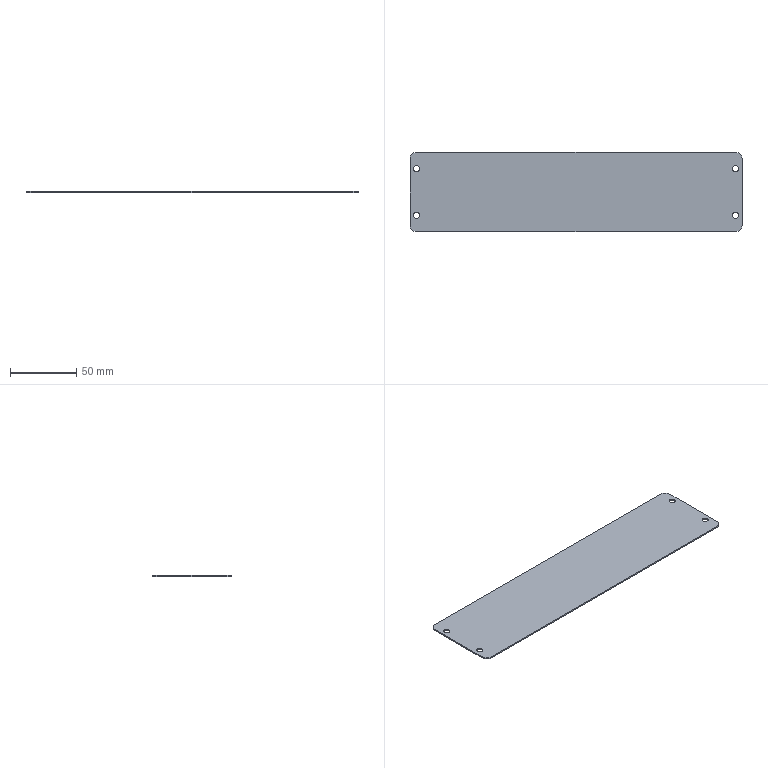Part | SolidWorks | features BreakCorner 1, FlatPattern 1, HoleWzd 1, SMBaseFlange 1, SheetMetal 1 | 1 solid | 18 faces | box 250 x 60 x 1 mm | volume 14915 mm3 | cylinder 12 | plane 6 | commonest cylinder face diameters 4.5 x8 10 x4
STEP:
#1=CARTESIAN_POINT('',(122.25,17.5,0.));
#2=VERTEX_POINT('',#1);
#3=CARTESIAN_POINT('',(117.75,17.5,0.));
#4=VERTEX_POINT('',#3);
#5=CARTESIAN_POINT('',(120.,17.5,0.));
#6=DIRECTION('',(0.,0.,-1.));
#7=DIRECTION('',(-1.,0.,0.));
#8=AXIS2_PLACEMENT_3D('',#5,#6,#7);
#9=CIRCLE('',#8,2.25);
#10=EDGE_CURVE('',#2,#4,#9,.T.);
#11=ORIENTED_EDGE('',*,*,#10,.F.);
#12=CARTESIAN_POINT('',(122.25,17.5,-1.));
#13=VERTEX_POINT('',#12);
#14=CARTESIAN_POINT('',(122.25,17.5,-1.));
#15=DIRECTION('',(0.,0.,-1.));
#16=VECTOR('',#15,1000.);
#17=LINE('',#14,#16);
#18=EDGE_CURVE('',#2,#13,#17,.T.);
#19=ORIENTED_EDGE('',*,*,#18,.T.);
#20=CARTESIAN_POINT('',(117.75,17.5,-1.));
#21=VERTEX_POINT('',#20);
#22=CARTESIAN_POINT('',(120.,17.5,-1.));
#23=DIRECTION('',(0.,0.,-1.));
#24=DIRECTION('',(-1.,0.,0.));
#25=AXIS2_PLACEMENT_3D('',#22,#23,#24);
#26=CIRCLE('',#25,2.25);
#27=EDGE_CURVE('',#13,#21,#26,.T.);
#28=ORIENTED_EDGE('',*,*,#27,.T.);
#29=CARTESIAN_POINT('',(117.75,17.5,-1.));
#30=DIRECTION('',(0.,0.,-1.));
#31=VECTOR('',#30,1000.);
#32=LINE('',#29,#31);
#33=EDGE_CURVE('',#4,#21,#32,.T.);
#34=ORIENTED_EDGE('',*,*,#33,.F.);
#35=EDGE_LOOP('',(#11,#19,#28,#34));
#36=FACE_OUTER_BOUND('',#35,.T.);
#37=CARTESIAN_POINT('',(120.,17.5,-1.));
#38=DIRECTION('',(0.,0.,-1.));
#39=DIRECTION('',(-1.,0.,0.));
#40=AXIS2_PLACEMENT_3D('',#37,#38,#39);
#41=CYLINDRICAL_SURFACE('',#40,2.25);
#42=ADVANCED_FACE('',(#36),#41,.F.);
#43=CARTESIAN_POINT('',(122.25,-17.5,0.));
#44=VERTEX_POINT('',#43);
#45=CARTESIAN_POINT('',(117.75,-17.5,0.));
#46=VERTEX_POINT('',#45);
#47=CARTESIAN_POINT('',(120.,-17.5,0.));
#48=DIRECTION('',(0.,0.,-1.));
#49=DIRECTION('',(-1.,0.,0.));
#50=AXIS2_PLACEMENT_3D('',#47,#48,#49);
#51=CIRCLE('',#50,2.25);
#52=EDGE_CURVE('',#44,#46,#51,.T.);
#53=ORIENTED_EDGE('',*,*,#52,.F.);
#54=CARTESIAN_POINT('',(122.25,-17.5,-1.));
#55=VERTEX_POINT('',#54);
#56=CARTESIAN_POINT('',(122.25,-17.5,-1.));
#57=DIRECTION('',(0.,0.,-1.));
#58=VECTOR('',#57,1000.);
#59=LINE('',#56,#58);
#60=EDGE_CURVE('',#44,#55,#59,.T.);
#61=ORIENTED_EDGE('',*,*,#60,.T.);
#62=CARTESIAN_POINT('',(117.75,-17.5,-1.));
#63=VERTEX_POINT('',#62);
#64=CARTESIAN_POINT('',(120.,-17.5,-1.));
#65=DIRECTION('',(0.,0.,-1.));
#66=DIRECTION('',(-1.,0.,0.));
#67=AXIS2_PLACEMENT_3D('',#64,#65,#66);
#68=CIRCLE('',#67,2.25);
#69=EDGE_CURVE('',#55,#63,#68,.T.);
#70=ORIENTED_EDGE('',*,*,#69,.T.);
#71=CARTESIAN_POINT('',(117.75,-17.5,-1.));
#72=DIRECTION('',(0.,0.,-1.));
#73=VECTOR('',#72,1000.);
#74=LINE('',#71,#73);
#75=EDGE_CURVE('',#46,#63,#74,.T.);
#76=ORIENTED_EDGE('',*,*,#75,.F.);
#77=EDGE_LOOP('',(#53,#61,#70,#76));
#78=FACE_OUTER_BOUND('',#77,.T.);
#79=CARTESIAN_POINT('',(120.,-17.5,-1.));
#80=DIRECTION('',(0.,0.,-1.));
#81=DIRECTION('',(-1.,0.,0.));
#82=AXIS2_PLACEMENT_3D('',#79,#80,#81);
#83=CYLINDRICAL_SURFACE('',#82,2.25);
#84=ADVANCED_FACE('',(#78),#83,.F.);
#85=CARTESIAN_POINT('',(-117.75,17.5,0.));
#86=VERTEX_POINT('',#85);
#87=CARTESIAN_POINT('',(-122.25,17.5,0.));
#88=VERTEX_POINT('',#87);
#89=CARTESIAN_POINT('',(-120.,17.5,0.));
#90=DIRECTION('',(0.,0.,-1.));
#91=DIRECTION('',(-1.,0.,0.));
#92=AXIS2_PLACEMENT_3D('',#89,#90,#91);
#93=CIRCLE('',#92,2.25);
#94=EDGE_CURVE('',#86,#88,#93,.T.);
#95=ORIENTED_EDGE('',*,*,#94,.F.);
#96=CARTESIAN_POINT('',(-117.75,17.5,-1.));
#97=VERTEX_POINT('',#96);
#98=CARTESIAN_POINT('',(-117.75,17.5,-1.));
#99=DIRECTION('',(0.,0.,-1.));
#100=VECTOR('',#99,1000.);
#101=LINE('',#98,#100);
#102=EDGE_CURVE('',#86,#97,#101,.T.);
#103=ORIENTED_EDGE('',*,*,#102,.T.);
#104=CARTESIAN_POINT('',(-122.25,17.5,-1.));
#105=VERTEX_POINT('',#104);
#106=CARTESIAN_POINT('',(-120.,17.5,-1.));
#107=DIRECTION('',(0.,0.,-1.));
#108=DIRECTION('',(-1.,0.,0.));
#109=AXIS2_PLACEMENT_3D('',#106,#107,#108);
#110=CIRCLE('',#109,2.25);
#111=EDGE_CURVE('',#97,#105,#110,.T.);
#112=ORIENTED_EDGE('',*,*,#111,.T.);
#113=CARTESIAN_POINT('',(-122.25,17.5,-1.));
#114=DIRECTION('',(0.,0.,-1.));
#115=VECTOR('',#114,1000.);
#116=LINE('',#113,#115);
#117=EDGE_CURVE('',#88,#105,#116,.T.);
#118=ORIENTED_EDGE('',*,*,#117,.F.);
#119=EDGE_LOOP('',(#95,#103,#112,#118));
#120=FACE_OUTER_BOUND('',#119,.T.);
#121=CARTESIAN_POINT('',(-120.,17.5,-1.));
#122=DIRECTION('',(0.,0.,-1.));
#123=DIRECTION('',(-1.,0.,0.));
#124=AXIS2_PLACEMENT_3D('',#121,#122,#123);
#125=CYLINDRICAL_SURFACE('',#124,2.25);
#126=ADVANCED_FACE('',(#120),#125,.F.);
#127=CARTESIAN_POINT('',(-117.75,-17.5,0.));
#128=VERTEX_POINT('',#127);
#129=CARTESIAN_POINT('',(-122.25,-17.5,0.));
#130=VERTEX_POINT('',#129);
#131=CARTESIAN_POINT('',(-120.,-17.5,0.));
#132=DIRECTION('',(0.,0.,-1.));
#133=DIRECTION('',(-1.,0.,0.));
#134=AXIS2_PLACEMENT_3D('',#131,#132,#133);
#135=CIRCLE('',#134,2.25);
#136=EDGE_CURVE('',#128,#130,#135,.T.);
#137=ORIENTED_EDGE('',*,*,#136,.F.);
#138=CARTESIAN_POINT('',(-117.75,-17.5,-1.));
#139=VERTEX_POINT('',#138);
#140=CARTESIAN_POINT('',(-117.75,-17.5,-1.));
#141=DIRECTION('',(0.,0.,-1.));
#142=VECTOR('',#141,1000.);
#143=LINE('',#140,#142);
#144=EDGE_CURVE('',#128,#139,#143,.T.);
#145=ORIENTED_EDGE('',*,*,#144,.T.);
#146=CARTESIAN_POINT('',(-122.25,-17.5,-1.));
#147=VERTEX_POINT('',#146);
#148=CARTESIAN_POINT('',(-120.,-17.5,-1.));
#149=DIRECTION('',(0.,0.,-1.));
#150=DIRECTION('',(-1.,0.,0.));
#151=AXIS2_PLACEMENT_3D('',#148,#149,#150);
#152=CIRCLE('',#151,2.25);
#153=EDGE_CURVE('',#139,#147,#152,.T.);
#154=ORIENTED_EDGE('',*,*,#153,.T.);
#155=CARTESIAN_POINT('',(-122.25,-17.5,-1.));
#156=DIRECTION('',(0.,0.,-1.));
#157=VECTOR('',#156,1000.);
#158=LINE('',#155,#157);
#159=EDGE_CURVE('',#130,#147,#158,.T.);
#160=ORIENTED_EDGE('',*,*,#159,.F.);
#161=EDGE_LOOP('',(#137,#145,#154,#160));
#162=FACE_OUTER_BOUND('',#161,.T.);
#163=CARTESIAN_POINT('',(-120.,-17.5,-1.));
#164=DIRECTION('',(0.,0.,-1.));
#165=DIRECTION('',(-1.,0.,0.));
#166=AXIS2_PLACEMENT_3D('',#163,#164,#165);
#167=CYLINDRICAL_SURFACE('',#166,2.25);
#168=ADVANCED_FACE('',(#162),#167,.F.);
#169=CARTESIAN_POINT('',(125.,-25.,-1.));
#170=VERTEX_POINT('',#169);
#171=CARTESIAN_POINT('',(125.,25.,-1.));
#172=VERTEX_POINT('',#171);
#173=CARTESIAN_POINT('',(125.,-30.,-1.));
#174=DIRECTION('',(0.,1.,0.));
#175=VECTOR('',#174,1000.);
#176=LINE('',#173,#175);
#177=EDGE_CURVE('',#170,#172,#176,.T.);
#178=ORIENTED_EDGE('',*,*,#177,.T.);
#179=CARTESIAN_POINT('',(125.,25.,0.));
#180=VERTEX_POINT('',#179);
#181=CARTESIAN_POINT('',(125.,25.,-1.));
#182=DIRECTION('',(0.,0.,1.));
#183=VECTOR('',#182,1000.);
#184=LINE('',#181,#183);
#185=EDGE_CURVE('',#172,#180,#184,.T.);
#186=ORIENTED_EDGE('',*,*,#185,.T.);
#187=CARTESIAN_POINT('',(125.,-25.,0.));
#188=VERTEX_POINT('',#187);
#189=CARTESIAN_POINT('',(125.,-30.,0.));
#190=DIRECTION('',(0.,1.,0.));
#191=VECTOR('',#190,1000.);
#192=LINE('',#189,#191);
#193=EDGE_CURVE('',#188,#180,#192,.T.);
#194=ORIENTED_EDGE('',*,*,#193,.F.);
#195=CARTESIAN_POINT('',(125.,-25.,-1.));
#196=DIRECTION('',(0.,0.,-1.));
#197=VECTOR('',#196,1000.);
#198=LINE('',#195,#197);
#199=EDGE_CURVE('',#188,#170,#198,.T.);
#200=ORIENTED_EDGE('',*,*,#199,.T.);
#201=EDGE_LOOP('',(#178,#186,#194,#200));
#202=FACE_OUTER_BOUND('',#201,.T.);
#203=CARTESIAN_POINT('',(125.,-30.,-1.));
#204=DIRECTION('',(1.,0.,0.));
#205=DIRECTION('',(0.,0.,-1.));
#206=AXIS2_PLACEMENT_3D('',#203,#204,#205);
#207=PLANE('',#206);
#208=ADVANCED_FACE('',(#202),#207,.T.);
#209=CARTESIAN_POINT('',(-120.,-30.,0.));
#210=VERTEX_POINT('',#209);
#211=CARTESIAN_POINT('',(120.,-30.,0.));
#212=VERTEX_POINT('',#211);
#213=CARTESIAN_POINT('',(-125.,-30.,0.));
#214=DIRECTION('',(1.,0.,0.));
#215=VECTOR('',#214,1000.);
#216=LINE('',#213,#215);
#217=EDGE_CURVE('',#210,#212,#216,.T.);
#218=ORIENTED_EDGE('',*,*,#217,.F.);
#219=CARTESIAN_POINT('',(-120.,-30.,-1.));
#220=VERTEX_POINT('',#219);
#221=CARTESIAN_POINT('',(-120.,-30.,-1.));
#222=DIRECTION('',(0.,0.,-1.));
#223=VECTOR('',#222,1000.);
#224=LINE('',#221,#223);
#225=EDGE_CURVE('',#210,#220,#224,.T.);
#226=ORIENTED_EDGE('',*,*,#225,.T.);
#227=CARTESIAN_POINT('',(120.,-30.,-1.));
#228=VERTEX_POINT('',#227);
#229=CARTESIAN_POINT('',(-125.,-30.,-1.));
#230=DIRECTION('',(1.,0.,0.));
#231=VECTOR('',#230,1000.);
#232=LINE('',#229,#231);
#233=EDGE_CURVE('',#220,#228,#232,.T.);
#234=ORIENTED_EDGE('',*,*,#233,.T.);
#235=CARTESIAN_POINT('',(120.,-30.,-1.));
#236=DIRECTION('',(0.,0.,1.));
#237=VECTOR('',#236,1000.);
#238=LINE('',#235,#237);
#239=EDGE_CURVE('',#228,#212,#238,.T.);
#240=ORIENTED_EDGE('',*,*,#239,.T.);
#241=EDGE_LOOP('',(#218,#226,#234,#240));
#242=FACE_OUTER_BOUND('',#241,.T.);
#243=CARTESIAN_POINT('',(-125.,-30.,-1.));
#244=DIRECTION('',(0.,-1.,0.));
#245=DIRECTION('',(0.,0.,-1.));
#246=AXIS2_PLACEMENT_3D('',#243,#244,#245);
#247=PLANE('',#246);
#248=ADVANCED_FACE('',(#242),#247,.T.);
#249=CARTESIAN_POINT('',(-125.,25.,0.));
#250=VERTEX_POINT('',#249);
#251=CARTESIAN_POINT('',(-125.,-25.,0.));
#252=VERTEX_POINT('',#251);
#253=CARTESIAN_POINT('',(-125.,-30.,0.));
#254=DIRECTION('',(0.,-1.,0.));
#255=VECTOR('',#254,1000.);
#256=LINE('',#253,#255);
#257=EDGE_CURVE('',#250,#252,#256,.T.);
#258=ORIENTED_EDGE('',*,*,#257,.F.);
#259=CARTESIAN_POINT('',(-125.,25.,-1.));
#260=VERTEX_POINT('',#259);
#261=CARTESIAN_POINT('',(-125.,25.,-1.));
#262=DIRECTION('',(0.,0.,-1.));
#263=VECTOR('',#262,1000.);
#264=LINE('',#261,#263);
#265=EDGE_CURVE('',#250,#260,#264,.T.);
#266=ORIENTED_EDGE('',*,*,#265,.T.);
#267=CARTESIAN_POINT('',(-125.,-25.,-1.));
#268=VERTEX_POINT('',#267);
#269=CARTESIAN_POINT('',(-125.,-30.,-1.));
#270=DIRECTION('',(0.,-1.,0.));
#271=VECTOR('',#270,1000.);
#272=LINE('',#269,#271);
#273=EDGE_CURVE('',#260,#268,#272,.T.);
#274=ORIENTED_EDGE('',*,*,#273,.T.);
#275=CARTESIAN_POINT('',(-125.,-25.,-1.));
#276=DIRECTION('',(0.,0.,1.));
#277=VECTOR('',#276,1000.);
#278=LINE('',#275,#277);
#279=EDGE_CURVE('',#268,#252,#278,.T.);
#280=ORIENTED_EDGE('',*,*,#279,.T.);
#281=EDGE_LOOP('',(#258,#266,#274,#280));
#282=FACE_OUTER_BOUND('',#281,.T.);
#283=CARTESIAN_POINT('',(-125.,-30.,-1.));
#284=DIRECTION('',(-1.,0.,0.));
#285=DIRECTION('',(0.,0.,1.));
#286=AXIS2_PLACEMENT_3D('',#283,#284,#285);
#287=PLANE('',#286);
#288=ADVANCED_FACE('',(#282),#287,.T.);
#289=CARTESIAN_POINT('',(120.,30.,0.));
#290=VERTEX_POINT('',#289);
#291=CARTESIAN_POINT('',(-120.,30.,0.));
#292=VERTEX_POINT('',#291);
#293=CARTESIAN_POINT('',(-125.,30.,0.));
#294=DIRECTION('',(-1.,0.,0.));
#295=VECTOR('',#294,1000.);
#296=LINE('',#293,#295);
#297=EDGE_CURVE('',#290,#292,#296,.T.);
#298=ORIENTED_EDGE('',*,*,#297,.F.);
#299=CARTESIAN_POINT('',(120.,30.,-1.));
#300=VERTEX_POINT('',#299);
#301=CARTESIAN_POINT('',(120.,30.,-1.));
#302=DIRECTION('',(0.,0.,-1.));
#303=VECTOR('',#302,1000.);
#304=LINE('',#301,#303);
#305=EDGE_CURVE('',#290,#300,#304,.T.);
#306=ORIENTED_EDGE('',*,*,#305,.T.);
#307=CARTESIAN_POINT('',(-120.,30.,-1.));
#308=VERTEX_POINT('',#307);
#309=CARTESIAN_POINT('',(-125.,30.,-1.));
#310=DIRECTION('',(-1.,0.,0.));
#311=VECTOR('',#310,1000.);
#312=LINE('',#309,#311);
#313=EDGE_CURVE('',#300,#308,#312,.T.);
#314=ORIENTED_EDGE('',*,*,#313,.T.);
#315=CARTESIAN_POINT('',(-120.,30.,-1.));
#316=DIRECTION('',(0.,0.,1.));
#317=VECTOR('',#316,1000.);
#318=LINE('',#315,#317);
#319=EDGE_CURVE('',#308,#292,#318,.T.);
#320=ORIENTED_EDGE('',*,*,#319,.T.);
#321=EDGE_LOOP('',(#298,#306,#314,#320));
#322=FACE_OUTER_BOUND('',#321,.T.);
#323=CARTESIAN_POINT('',(-125.,30.,-1.));
#324=DIRECTION('',(0.,1.,0.));
#325=DIRECTION('',(0.,0.,1.));
#326=AXIS2_PLACEMENT_3D('',#323,#324,#325);
#327=PLANE('',#326);
#328=ADVANCED_FACE('',(#322),#327,.T.);
#329=CARTESIAN_POINT('',(120.,17.5,-1.));
#330=DIRECTION('',(0.,0.,-1.));
#331=DIRECTION('',(-1.,0.,0.));
#332=AXIS2_PLACEMENT_3D('',#329,#330,#331);
#333=CIRCLE('',#332,2.25);
#334=EDGE_CURVE('',#21,#13,#333,.T.);
#335=ORIENTED_EDGE('',*,*,#334,.F.);
#336=ORIENTED_EDGE('',*,*,#27,.F.);
#337=EDGE_LOOP('',(#335,#336));
#338=FACE_BOUND('',#337,.T.);
#339=CARTESIAN_POINT('',(120.,-17.5,-1.));
#340=DIRECTION('',(0.,0.,-1.));
#341=DIRECTION('',(-1.,0.,0.));
#342=AXIS2_PLACEMENT_3D('',#339,#340,#341);
#343=CIRCLE('',#342,2.25);
#344=EDGE_CURVE('',#63,#55,#343,.T.);
#345=ORIENTED_EDGE('',*,*,#344,.F.);
#346=ORIENTED_EDGE('',*,*,#69,.F.);
#347=EDGE_LOOP('',(#345,#346));
#348=FACE_BOUND('',#347,.T.);
#349=CARTESIAN_POINT('',(-120.,17.5,-1.));
#350=DIRECTION('',(0.,0.,-1.));
#351=DIRECTION('',(-1.,0.,0.));
#352=AXIS2_PLACEMENT_3D('',#349,#350,#351);
#353=CIRCLE('',#352,2.25);
#354=EDGE_CURVE('',#105,#97,#353,.T.);
#355=ORIENTED_EDGE('',*,*,#354,.F.);
#356=ORIENTED_EDGE('',*,*,#111,.F.);
#357=EDGE_LOOP('',(#355,#356));
#358=FACE_BOUND('',#357,.T.);
#359=CARTESIAN_POINT('',(-120.,-17.5,-1.));
#360=DIRECTION('',(0.,0.,-1.));
#361=DIRECTION('',(-1.,0.,0.));
#362=AXIS2_PLACEMENT_3D('',#359,#360,#361);
#363=CIRCLE('',#362,2.25);
#364=EDGE_CURVE('',#147,#139,#363,.T.);
#365=ORIENTED_EDGE('',*,*,#364,.F.);
#366=ORIENTED_EDGE('',*,*,#153,.F.);
#367=EDGE_LOOP('',(#365,#366));
#368=FACE_BOUND('',#367,.T.);
#369=ORIENTED_EDGE('',*,*,#313,.F.);
#370=CARTESIAN_POINT('',(120.,25.,-1.));
#371=DIRECTION('',(0.,0.,-1.));
#372=DIRECTION('',(-1.,0.,0.));
#373=AXIS2_PLACEMENT_3D('',#370,#371,#372);
#374=CIRCLE('',#373,5.);
#375=EDGE_CURVE('',#300,#172,#374,.T.);
#376=ORIENTED_EDGE('',*,*,#375,.T.);
#377=ORIENTED_EDGE('',*,*,#177,.F.);
#378=CARTESIAN_POINT('',(120.,-25.,-1.));
#379=DIRECTION('',(0.,0.,-1.));
#380=DIRECTION('',(-1.,0.,0.));
#381=AXIS2_PLACEMENT_3D('',#378,#379,#380);
#382=CIRCLE('',#381,5.);
#383=EDGE_CURVE('',#170,#228,#382,.T.);
#384=ORIENTED_EDGE('',*,*,#383,.T.);
#385=ORIENTED_EDGE('',*,*,#233,.F.);
#386=CARTESIAN_POINT('',(-120.,-25.,-1.));
#387=DIRECTION('',(0.,0.,-1.));
#388=DIRECTION('',(-1.,0.,0.));
#389=AXIS2_PLACEMENT_3D('',#386,#387,#388);
#390=CIRCLE('',#389,5.);
#391=EDGE_CURVE('',#220,#268,#390,.T.);
#392=ORIENTED_EDGE('',*,*,#391,.T.);
#393=ORIENTED_EDGE('',*,*,#273,.F.);
#394=CARTESIAN_POINT('',(-120.,25.,-1.));
#395=DIRECTION('',(0.,0.,-1.));
#396=DIRECTION('',(-1.,0.,0.));
#397=AXIS2_PLACEMENT_3D('',#394,#395,#396);
#398=CIRCLE('',#397,5.);
#399=EDGE_CURVE('',#260,#308,#398,.T.);
#400=ORIENTED_EDGE('',*,*,#399,.T.);
#401=EDGE_LOOP('',(#369,#376,#377,#384,#385,#392,#393,#400));
#402=FACE_OUTER_BOUND('',#401,.T.);
#403=CARTESIAN_POINT('',(0.,0.,-1.));
#404=DIRECTION('',(0.,0.,-1.));
#405=DIRECTION('',(-1.,0.,0.));
#406=AXIS2_PLACEMENT_3D('',#403,#404,#405);
#407=PLANE('',#406);
#408=ADVANCED_FACE('',(#338,#348,#358,#368,#402),#407,.T.);
#409=CARTESIAN_POINT('',(120.,17.5,0.));
#410=DIRECTION('',(0.,0.,-1.));
#411=DIRECTION('',(-1.,0.,0.));
#412=AXIS2_PLACEMENT_3D('',#409,#410,#411);
#413=CIRCLE('',#412,2.25);
#414=EDGE_CURVE('',#4,#2,#413,.T.);
#415=ORIENTED_EDGE('',*,*,#414,.T.);
#416=ORIENTED_EDGE('',*,*,#10,.T.);
#417=EDGE_LOOP('',(#415,#416));
#418=FACE_BOUND('',#417,.T.);
#419=CARTESIAN_POINT('',(120.,-17.5,0.));
#420=DIRECTION('',(0.,0.,-1.));
#421=DIRECTION('',(-1.,0.,0.));
#422=AXIS2_PLACEMENT_3D('',#419,#420,#421);
#423=CIRCLE('',#422,2.25);
#424=EDGE_CURVE('',#46,#44,#423,.T.);
#425=ORIENTED_EDGE('',*,*,#424,.T.);
#426=ORIENTED_EDGE('',*,*,#52,.T.);
#427=EDGE_LOOP('',(#425,#426));
#428=FACE_BOUND('',#427,.T.);
#429=CARTESIAN_POINT('',(-120.,17.5,0.));
#430=DIRECTION('',(0.,0.,-1.));
#431=DIRECTION('',(-1.,0.,0.));
#432=AXIS2_PLACEMENT_3D('',#429,#430,#431);
#433=CIRCLE('',#432,2.25);
#434=EDGE_CURVE('',#88,#86,#433,.T.);
#435=ORIENTED_EDGE('',*,*,#434,.T.);
#436=ORIENTED_EDGE('',*,*,#94,.T.);
#437=EDGE_LOOP('',(#435,#436));
#438=FACE_BOUND('',#437,.T.);
#439=CARTESIAN_POINT('',(-120.,-17.5,0.));
#440=DIRECTION('',(0.,0.,-1.));
#441=DIRECTION('',(-1.,0.,0.));
#442=AXIS2_PLACEMENT_3D('',#439,#440,#441);
#443=CIRCLE('',#442,2.25);
#444=EDGE_CURVE('',#130,#128,#443,.T.);
#445=ORIENTED_EDGE('',*,*,#444,.T.);
#446=ORIENTED_EDGE('',*,*,#136,.T.);
#447=EDGE_LOOP('',(#445,#446));
#448=FACE_BOUND('',#447,.T.);
#449=ORIENTED_EDGE('',*,*,#193,.T.);
#450=CARTESIAN_POINT('',(120.,25.,0.));
#451=DIRECTION('',(0.,0.,1.));
#452=DIRECTION('',(-1.,0.,0.));
#453=AXIS2_PLACEMENT_3D('',#450,#451,#452);
#454=CIRCLE('',#453,5.);
#455=EDGE_CURVE('',#180,#290,#454,.T.);
#456=ORIENTED_EDGE('',*,*,#455,.T.);
#457=ORIENTED_EDGE('',*,*,#297,.T.);
#458=CARTESIAN_POINT('',(-120.,25.,0.));
#459=DIRECTION('',(0.,0.,1.));
#460=DIRECTION('',(-1.,0.,0.));
#461=AXIS2_PLACEMENT_3D('',#458,#459,#460);
#462=CIRCLE('',#461,5.);
#463=EDGE_CURVE('',#292,#250,#462,.T.);
#464=ORIENTED_EDGE('',*,*,#463,.T.);
#465=ORIENTED_EDGE('',*,*,#257,.T.);
#466=CARTESIAN_POINT('',(-120.,-25.,0.));
#467=DIRECTION('',(0.,0.,1.));
#468=DIRECTION('',(-1.,0.,0.));
#469=AXIS2_PLACEMENT_3D('',#466,#467,#468);
#470=CIRCLE('',#469,5.);
#471=EDGE_CURVE('',#252,#210,#470,.T.);
#472=ORIENTED_EDGE('',*,*,#471,.T.);
#473=ORIENTED_EDGE('',*,*,#217,.T.);
#474=CARTESIAN_POINT('',(120.,-25.,0.));
#475=DIRECTION('',(0.,0.,1.));
#476=DIRECTION('',(-1.,0.,0.));
#477=AXIS2_PLACEMENT_3D('',#474,#475,#476);
#478=CIRCLE('',#477,5.);
#479=EDGE_CURVE('',#212,#188,#478,.T.);
#480=ORIENTED_EDGE('',*,*,#479,.T.);
#481=EDGE_LOOP('',(#449,#456,#457,#464,#465,#472,#473,#480));
#482=FACE_OUTER_BOUND('',#481,.T.);
#483=CARTESIAN_POINT('',(0.,0.,0.));
#484=DIRECTION('',(0.,0.,-1.));
#485=DIRECTION('',(-1.,0.,0.));
#486=AXIS2_PLACEMENT_3D('',#483,#484,#485);
#487=PLANE('',#486);
#488=ADVANCED_FACE('',(#418,#428,#438,#448,#482),#487,.F.);
#489=ORIENTED_EDGE('',*,*,#144,.F.);
#490=ORIENTED_EDGE('',*,*,#444,.F.);
#491=ORIENTED_EDGE('',*,*,#159,.T.);
#492=ORIENTED_EDGE('',*,*,#364,.T.);
#493=EDGE_LOOP('',(#489,#490,#491,#492));
#494=FACE_OUTER_BOUND('',#493,.T.);
#495=CARTESIAN_POINT('',(-120.,-17.5,-1.));
#496=DIRECTION('',(0.,0.,-1.));
#497=DIRECTION('',(-1.,0.,0.));
#498=AXIS2_PLACEMENT_3D('',#495,#496,#497);
#499=CYLINDRICAL_SURFACE('',#498,2.25);
#500=ADVANCED_FACE('',(#494),#499,.F.);
#501=ORIENTED_EDGE('',*,*,#102,.F.);
#502=ORIENTED_EDGE('',*,*,#434,.F.);
#503=ORIENTED_EDGE('',*,*,#117,.T.);
#504=ORIENTED_EDGE('',*,*,#354,.T.);
#505=EDGE_LOOP('',(#501,#502,#503,#504));
#506=FACE_OUTER_BOUND('',#505,.T.);
#507=CARTESIAN_POINT('',(-120.,17.5,-1.));
#508=DIRECTION('',(0.,0.,-1.));
#509=DIRECTION('',(-1.,0.,0.));
#510=AXIS2_PLACEMENT_3D('',#507,#508,#509);
#511=CYLINDRICAL_SURFACE('',#510,2.25);
#512=ADVANCED_FACE('',(#506),#511,.F.);
#513=ORIENTED_EDGE('',*,*,#60,.F.);
#514=ORIENTED_EDGE('',*,*,#424,.F.);
#515=ORIENTED_EDGE('',*,*,#75,.T.);
#516=ORIENTED_EDGE('',*,*,#344,.T.);
#517=EDGE_LOOP('',(#513,#514,#515,#516));
#518=FACE_OUTER_BOUND('',#517,.T.);
#519=CARTESIAN_POINT('',(120.,-17.5,-1.));
#520=DIRECTION('',(0.,0.,-1.));
#521=DIRECTION('',(-1.,0.,0.));
#522=AXIS2_PLACEMENT_3D('',#519,#520,#521);
#523=CYLINDRICAL_SURFACE('',#522,2.25);
#524=ADVANCED_FACE('',(#518),#523,.F.);
#525=ORIENTED_EDGE('',*,*,#18,.F.);
#526=ORIENTED_EDGE('',*,*,#414,.F.);
#527=ORIENTED_EDGE('',*,*,#33,.T.);
#528=ORIENTED_EDGE('',*,*,#334,.T.);
#529=EDGE_LOOP('',(#525,#526,#527,#528));
#530=FACE_OUTER_BOUND('',#529,.T.);
#531=CARTESIAN_POINT('',(120.,17.5,-1.));
#532=DIRECTION('',(0.,0.,-1.));
#533=DIRECTION('',(-1.,0.,0.));
#534=AXIS2_PLACEMENT_3D('',#531,#532,#533);
#535=CYLINDRICAL_SURFACE('',#534,2.25);
#536=ADVANCED_FACE('',(#530),#535,.F.);
#537=ORIENTED_EDGE('',*,*,#375,.F.);
#538=ORIENTED_EDGE('',*,*,#305,.F.);
#539=ORIENTED_EDGE('',*,*,#455,.F.);
#540=ORIENTED_EDGE('',*,*,#185,.F.);
#541=EDGE_LOOP('',(#537,#538,#539,#540));
#542=FACE_OUTER_BOUND('',#541,.T.);
#543=CARTESIAN_POINT('',(120.,25.,-1.));
#544=DIRECTION('',(0.,0.,1.));
#545=DIRECTION('',(1.,0.,0.));
#546=AXIS2_PLACEMENT_3D('',#543,#544,#545);
#547=CYLINDRICAL_SURFACE('',#546,5.);
#548=ADVANCED_FACE('',(#542),#547,.T.);
#549=ORIENTED_EDGE('',*,*,#399,.F.);
#550=ORIENTED_EDGE('',*,*,#265,.F.);
#551=ORIENTED_EDGE('',*,*,#463,.F.);
#552=ORIENTED_EDGE('',*,*,#319,.F.);
#553=EDGE_LOOP('',(#549,#550,#551,#552));
#554=FACE_OUTER_BOUND('',#553,.T.);
#555=CARTESIAN_POINT('',(-120.,25.,-1.));
#556=DIRECTION('',(0.,0.,1.));
#557=DIRECTION('',(1.,0.,0.));
#558=AXIS2_PLACEMENT_3D('',#555,#556,#557);
#559=CYLINDRICAL_SURFACE('',#558,5.);
#560=ADVANCED_FACE('',(#554),#559,.T.);
#561=ORIENTED_EDGE('',*,*,#391,.F.);
#562=ORIENTED_EDGE('',*,*,#225,.F.);
#563=ORIENTED_EDGE('',*,*,#471,.F.);
#564=ORIENTED_EDGE('',*,*,#279,.F.);
#565=EDGE_LOOP('',(#561,#562,#563,#564));
#566=FACE_OUTER_BOUND('',#565,.T.);
#567=CARTESIAN_POINT('',(-120.,-25.,-1.));
#568=DIRECTION('',(0.,0.,1.));
#569=DIRECTION('',(1.,0.,0.));
#570=AXIS2_PLACEMENT_3D('',#567,#568,#569);
#571=CYLINDRICAL_SURFACE('',#570,5.);
#572=ADVANCED_FACE('',(#566),#571,.T.);
#573=ORIENTED_EDGE('',*,*,#383,.F.);
#574=ORIENTED_EDGE('',*,*,#199,.F.);
#575=ORIENTED_EDGE('',*,*,#479,.F.);
#576=ORIENTED_EDGE('',*,*,#239,.F.);
#577=EDGE_LOOP('',(#573,#574,#575,#576));
#578=FACE_OUTER_BOUND('',#577,.T.);
#579=CARTESIAN_POINT('',(120.,-25.,-1.));
#580=DIRECTION('',(0.,0.,1.));
#581=DIRECTION('',(1.,0.,0.));
#582=AXIS2_PLACEMENT_3D('',#579,#580,#581);
#583=CYLINDRICAL_SURFACE('',#582,5.);
#584=ADVANCED_FACE('',(#578),#583,.T.);
#585=CLOSED_SHELL('',(#42,#84,#126,#168,#208,#248,#288,#328,#408,#488,#500,#512,#524,#536,#548,#560,#572,#584));
#586=MANIFOLD_SOLID_BREP('',#585);
#587=CARTESIAN_POINT('',(0.,0.,0.));
#588=DIRECTION('',(0.,0.,1.));
#589=DIRECTION('',(1.,0.,0.));
#590=AXIS2_PLACEMENT_3D('',#587,#588,#589);
#591=(LENGTH_UNIT()NAMED_UNIT(*)SI_UNIT(.MILLI.,.METRE.));
#592=UNCERTAINTY_MEASURE_WITH_UNIT(LENGTH_MEASURE(0.00001),#591,'','');
#593=(NAMED_UNIT(*)PLANE_ANGLE_UNIT()SI_UNIT($,.RADIAN.));
#594=(NAMED_UNIT(*)SI_UNIT($,.STERADIAN.)SOLID_ANGLE_UNIT());
#595=(GEOMETRIC_REPRESENTATION_CONTEXT(3)GLOBAL_UNCERTAINTY_ASSIGNED_CONTEXT((#592))GLOBAL_UNIT_ASSIGNED_CONTEXT((#591,#593,#594))REPRESENTATION_CONTEXT('',''));
#596=ADVANCED_BREP_SHAPE_REPRESENTATION('',(#586,#590),#595);